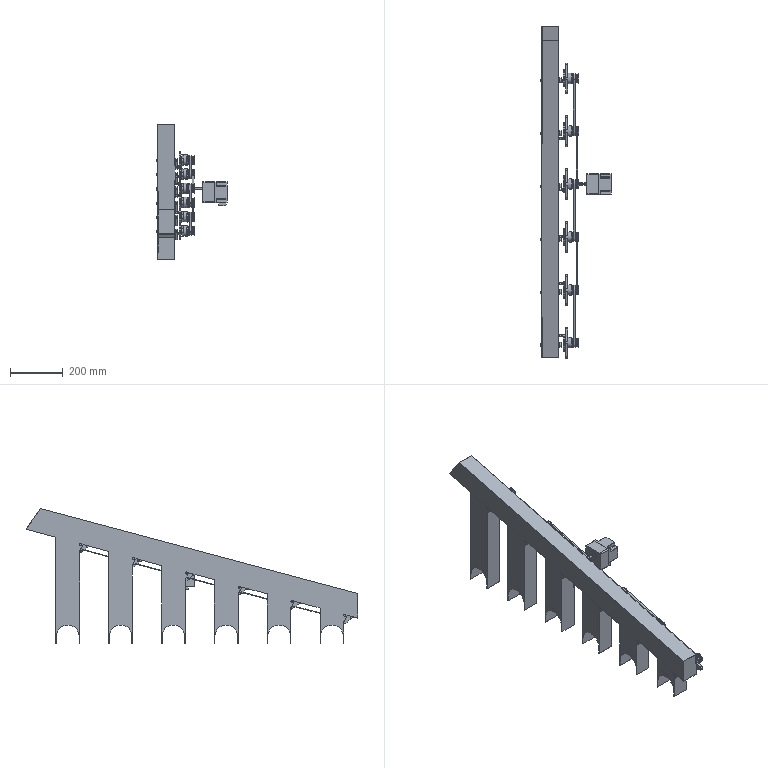Part | NX | features EXTRUDE 30, EXTRACT_STRING 18, Instance Feature 16, DATUM_CSYS 14, EXTRACT_FACE 14, SKETCH 9, BREP 7, skf_bearing_4200_atn9_2_1 5, HOLE PACKAGE 3, Pattern Feature 3, FSET 2, MOVE_FACE 2, OFFSET_REGION 2, RECT_GROOVE 2, SIMPLE HOLE 2, SYMBOLIC_THREAD 2, CSUNK_HOLE 1, DIVIDE_FACE 1, FILLET_WELD 1, LINE 1, LINKED_CURVE 1, Mirror Feature 1, SHELL 1, WELD_GROOVE 1 | 127 solids | 5715 faces | volume 2656651 mm3 | cylinder 3854 | plane 1465 | cone 162 | torus 144 | sphere 84 | spline 6 | commonest cylinder face diameters 0.3 x828 0.56 x816 3.95 x816 27.58 x408 29.8 x396 10 x73